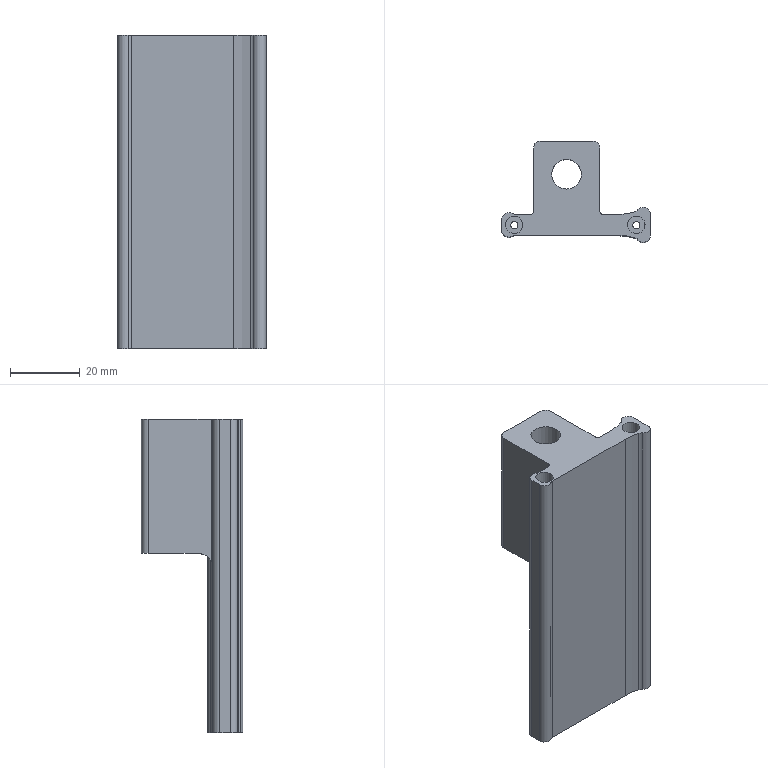Part | NX | features PU-13 2 | 1 solid | 34 faces | box 42.598 x 29.017 x 90 mm | volume 33900 mm3 | cylinder 19 | plane 13 | spline 2 | commonest cylinder face diameters 4 x10 2 x2 2.101 x2 5 x2 8.506 x1 10 x1
STEP:
#1=CARTESIAN_POINT('',(3882.334,-855.122,945.716));
#2=VERTEX_POINT('',#1);
#3=CARTESIAN_POINT('',(3882.334,-855.122,902.217));
#4=VERTEX_POINT('',#3);
#5=CARTESIAN_POINT('',(3882.334,-855.122,935.716));
#6=DIRECTION('',(0.,0.,-1.));
#7=VECTOR('',#6,1000.);
#8=LINE('',#5,#7);
#9=EDGE_CURVE('',#2,#4,#8,.T.);
#10=ORIENTED_EDGE('',*,*,#9,.T.);
#11=CARTESIAN_POINT('',(3903.334,-855.122,902.217));
#12=VERTEX_POINT('',#11);
#13=CARTESIAN_POINT('',(3903.334,-855.122,902.217));
#14=DIRECTION('',(-1.,0.,0.));
#15=VECTOR('',#14,1000.);
#16=LINE('',#13,#15);
#17=EDGE_CURVE('',#4,#12,#16,.F.);
#18=ORIENTED_EDGE('',*,*,#17,.T.);
#19=CARTESIAN_POINT('',(3903.334,-855.122,945.716));
#20=VERTEX_POINT('',#19);
#21=CARTESIAN_POINT('',(3903.334,-855.122,935.716));
#22=DIRECTION('',(0.,0.,-1.));
#23=VECTOR('',#22,1000.);
#24=LINE('',#21,#23);
#25=EDGE_CURVE('',#12,#20,#24,.F.);
#26=ORIENTED_EDGE('',*,*,#25,.T.);
#27=CARTESIAN_POINT('',(3907.495,-855.122,945.716));
#28=VERTEX_POINT('',#27);
#29=CARTESIAN_POINT('',(3897.665,-855.122,945.716));
#30=DIRECTION('',(1.,0.,0.));
#31=VECTOR('',#30,1000.);
#32=LINE('',#29,#31);
#33=EDGE_CURVE('',#20,#28,#32,.T.);
#34=ORIENTED_EDGE('',*,*,#33,.T.);
#35=CARTESIAN_POINT('',(3907.495,-855.122,855.716));
#36=VERTEX_POINT('',#35);
#37=CARTESIAN_POINT('',(3907.495,-855.122,945.716));
#38=CARTESIAN_POINT('',(3907.495,-855.122,915.716));
#39=CARTESIAN_POINT('',(3907.495,-855.122,885.716));
#40=CARTESIAN_POINT('',(3907.495,-855.122,855.716));
#41=B_SPLINE_CURVE_WITH_KNOTS('',3,(#37,#38,#39,#40),.UNSPECIFIED.,.F.,.F.,(4,4),(-0.125,1.),.UNSPECIFIED.);
#42=EDGE_CURVE('',#28,#36,#41,.T.);
#43=ORIENTED_EDGE('',*,*,#42,.T.);
#44=CARTESIAN_POINT('',(3878.173,-855.122,855.716));
#45=VERTEX_POINT('',#44);
#46=CARTESIAN_POINT('',(3897.665,-855.122,855.716));
#47=DIRECTION('',(1.,0.,0.));
#48=VECTOR('',#47,1000.);
#49=LINE('',#46,#48);
#50=EDGE_CURVE('',#36,#45,#49,.F.);
#51=ORIENTED_EDGE('',*,*,#50,.T.);
#52=CARTESIAN_POINT('',(3878.173,-855.122,945.716));
#53=VERTEX_POINT('',#52);
#54=CARTESIAN_POINT('',(3878.173,-855.122,935.716));
#55=DIRECTION('',(0.,0.,-1.));
#56=VECTOR('',#55,1000.);
#57=LINE('',#54,#56);
#58=EDGE_CURVE('',#53,#45,#57,.T.);
#59=ORIENTED_EDGE('',*,*,#58,.F.);
#60=CARTESIAN_POINT('',(3897.665,-855.122,945.716));
#61=DIRECTION('',(1.,0.,0.));
#62=VECTOR('',#61,1000.);
#63=LINE('',#60,#62);
#64=EDGE_CURVE('',#53,#2,#63,.T.);
#65=ORIENTED_EDGE('',*,*,#64,.T.);
#66=EDGE_LOOP('',(#10,#18,#26,#34,#43,#51,#59,#65));
#67=FACE_BOUND('',#66,.T.);
#68=CARTESIAN_POINT('',(3892.84,-855.122,895.716));
#69=DIRECTION('',(0.,1.,0.));
#70=DIRECTION('',(0.,0.,1.));
#71=AXIS2_PLACEMENT_3D('',#68,#69,#70);
#72=PLANE('',#71);
#73=ADVANCED_FACE('',(#67),#72,.T.);
#74=CARTESIAN_POINT('',(3874.236,-856.622,855.716));
#75=VERTEX_POINT('',#74);
#76=CARTESIAN_POINT('',(3874.236,-859.622,855.716));
#77=VERTEX_POINT('',#76);
#78=CARTESIAN_POINT('',(3874.236,-859.622,855.716));
#79=DIRECTION('',(0.,-1.,0.));
#80=VECTOR('',#79,1000.);
#81=LINE('',#78,#80);
#82=EDGE_CURVE('',#75,#77,#81,.T.);
#83=ORIENTED_EDGE('',*,*,#82,.T.);
#84=CARTESIAN_POINT('',(3874.236,-859.622,945.716));
#85=VERTEX_POINT('',#84);
#86=CARTESIAN_POINT('',(3874.236,-859.622,935.716));
#87=DIRECTION('',(0.,0.,-1.));
#88=VECTOR('',#87,1000.);
#89=LINE('',#86,#88);
#90=EDGE_CURVE('',#85,#77,#89,.T.);
#91=ORIENTED_EDGE('',*,*,#90,.F.);
#92=CARTESIAN_POINT('',(3874.236,-856.622,945.716));
#93=VERTEX_POINT('',#92);
#94=CARTESIAN_POINT('',(3874.236,-859.622,945.716));
#95=DIRECTION('',(0.,-1.,0.));
#96=VECTOR('',#95,1000.);
#97=LINE('',#94,#96);
#98=EDGE_CURVE('',#93,#85,#97,.T.);
#99=ORIENTED_EDGE('',*,*,#98,.F.);
#100=CARTESIAN_POINT('',(3874.236,-856.622,945.716));
#101=CARTESIAN_POINT('',(3874.236,-856.622,915.716));
#102=CARTESIAN_POINT('',(3874.236,-856.622,885.716));
#103=CARTESIAN_POINT('',(3874.236,-856.622,855.716));
#104=B_SPLINE_CURVE_WITH_KNOTS('',3,(#100,#101,#102,#103),.UNSPECIFIED.,.F.,.F.,(4,4),(-0.125,1.),.UNSPECIFIED.);
#105=EDGE_CURVE('',#93,#75,#104,.T.);
#106=ORIENTED_EDGE('',*,*,#105,.T.);
#107=EDGE_LOOP('',(#83,#91,#99,#106));
#108=FACE_BOUND('',#107,.T.);
#109=CARTESIAN_POINT('',(3874.236,-859.622,935.716));
#110=DIRECTION('',(1.,0.,0.));
#111=DIRECTION('',(0.,0.,-1.));
#112=AXIS2_PLACEMENT_3D('',#109,#110,#111);
#113=PLANE('',#112);
#114=ADVANCED_FACE('',(#108),#113,.F.);
#115=CARTESIAN_POINT('',(3877.204,-861.372,855.716));
#116=VERTEX_POINT('',#115);
#117=CARTESIAN_POINT('',(3876.236,-859.622,855.716));
#118=DIRECTION('',(0.,0.,1.));
#119=DIRECTION('',(1.,0.,0.));
#120=AXIS2_PLACEMENT_3D('',#117,#118,#119);
#121=CIRCLE('',#120,2.);
#122=EDGE_CURVE('',#116,#77,#121,.F.);
#123=ORIENTED_EDGE('',*,*,#122,.F.);
#124=CARTESIAN_POINT('',(3877.204,-861.372,945.716));
#125=VERTEX_POINT('',#124);
#126=CARTESIAN_POINT('',(3877.204,-861.372,855.716));
#127=CARTESIAN_POINT('',(3877.204,-861.372,885.716));
#128=CARTESIAN_POINT('',(3877.204,-861.372,915.716));
#129=CARTESIAN_POINT('',(3877.204,-861.372,945.716));
#130=B_SPLINE_CURVE_WITH_KNOTS('',3,(#126,#127,#128,#129),.UNSPECIFIED.,.F.,.F.,(4,4),(0.,1.125),.UNSPECIFIED.);
#131=EDGE_CURVE('',#125,#116,#130,.F.);
#132=ORIENTED_EDGE('',*,*,#131,.F.);
#133=CARTESIAN_POINT('',(3876.236,-859.622,945.716));
#134=DIRECTION('',(0.,0.,1.));
#135=DIRECTION('',(1.,0.,0.));
#136=AXIS2_PLACEMENT_3D('',#133,#134,#135);
#137=CIRCLE('',#136,2.);
#138=EDGE_CURVE('',#125,#85,#137,.F.);
#139=ORIENTED_EDGE('',*,*,#138,.T.);
#140=ORIENTED_EDGE('',*,*,#90,.T.);
#141=EDGE_LOOP('',(#123,#132,#139,#140));
#142=FACE_BOUND('',#141,.T.);
#143=CARTESIAN_POINT('',(3876.236,-859.622,935.716));
#144=DIRECTION('',(0.,0.,-1.));
#145=DIRECTION('',(-1.,0.,0.));
#146=AXIS2_PLACEMENT_3D('',#143,#144,#145);
#147=CYLINDRICAL_SURFACE('',#146,2.);
#148=ADVANCED_FACE('',(#142),#147,.T.);
#149=CARTESIAN_POINT('',(3878.173,-861.122,855.716));
#150=VERTEX_POINT('',#149);
#151=CARTESIAN_POINT('',(3878.173,-863.122,855.716));
#152=DIRECTION('',(0.,0.,1.));
#153=DIRECTION('',(1.,0.,0.));
#154=AXIS2_PLACEMENT_3D('',#151,#152,#153);
#155=CIRCLE('',#154,2.);
#156=EDGE_CURVE('',#150,#116,#155,.T.);
#157=ORIENTED_EDGE('',*,*,#156,.F.);
#158=CARTESIAN_POINT('',(3878.173,-861.122,945.716));
#159=VERTEX_POINT('',#158);
#160=CARTESIAN_POINT('',(3878.173,-861.122,935.716));
#161=DIRECTION('',(0.,0.,-1.));
#162=VECTOR('',#161,1000.);
#163=LINE('',#160,#162);
#164=EDGE_CURVE('',#159,#150,#163,.T.);
#165=ORIENTED_EDGE('',*,*,#164,.F.);
#166=CARTESIAN_POINT('',(3878.173,-863.122,945.716));
#167=DIRECTION('',(0.,0.,1.));
#168=DIRECTION('',(1.,0.,0.));
#169=AXIS2_PLACEMENT_3D('',#166,#167,#168);
#170=CIRCLE('',#169,2.);
#171=EDGE_CURVE('',#159,#125,#170,.T.);
#172=ORIENTED_EDGE('',*,*,#171,.T.);
#173=ORIENTED_EDGE('',*,*,#131,.T.);
#174=EDGE_LOOP('',(#157,#165,#172,#173));
#175=FACE_BOUND('',#174,.T.);
#176=CARTESIAN_POINT('',(3878.173,-863.122,935.716));
#177=DIRECTION('',(0.,0.,-1.));
#178=DIRECTION('',(-1.,0.,0.));
#179=AXIS2_PLACEMENT_3D('',#176,#177,#178);
#180=CYLINDRICAL_SURFACE('',#179,2.);
#181=ADVANCED_FACE('',(#175),#180,.F.);
#182=CARTESIAN_POINT('',(3907.495,-861.122,855.716));
#183=VERTEX_POINT('',#182);
#184=CARTESIAN_POINT('',(3897.665,-861.122,855.716));
#185=DIRECTION('',(1.,0.,0.));
#186=VECTOR('',#185,1000.);
#187=LINE('',#184,#186);
#188=EDGE_CURVE('',#150,#183,#187,.T.);
#189=ORIENTED_EDGE('',*,*,#188,.T.);
#190=CARTESIAN_POINT('',(3907.495,-861.122,945.716));
#191=VERTEX_POINT('',#190);
#192=CARTESIAN_POINT('',(3907.495,-861.122,855.716));
#193=CARTESIAN_POINT('',(3907.495,-861.122,885.716));
#194=CARTESIAN_POINT('',(3907.495,-861.122,915.716));
#195=CARTESIAN_POINT('',(3907.495,-861.122,945.716));
#196=B_SPLINE_CURVE_WITH_KNOTS('',3,(#192,#193,#194,#195),.UNSPECIFIED.,.F.,.F.,(4,4),(0.,1.125),.UNSPECIFIED.);
#197=EDGE_CURVE('',#191,#183,#196,.F.);
#198=ORIENTED_EDGE('',*,*,#197,.F.);
#199=CARTESIAN_POINT('',(3897.665,-861.122,945.716));
#200=DIRECTION('',(1.,0.,0.));
#201=VECTOR('',#200,1000.);
#202=LINE('',#199,#201);
#203=EDGE_CURVE('',#159,#191,#202,.T.);
#204=ORIENTED_EDGE('',*,*,#203,.F.);
#205=ORIENTED_EDGE('',*,*,#164,.T.);
#206=EDGE_LOOP('',(#189,#198,#204,#205));
#207=FACE_BOUND('',#206,.T.);
#208=CARTESIAN_POINT('',(3897.665,-861.122,935.716));
#209=DIRECTION('',(0.,1.,0.));
#210=DIRECTION('',(-1.,0.,0.));
#211=AXIS2_PLACEMENT_3D('',#208,#209,#210);
#212=PLANE('',#211);
#213=ADVANCED_FACE('',(#207),#212,.F.);
#214=CARTESIAN_POINT('',(3912.373,-861.817,855.716));
#215=VERTEX_POINT('',#214);
#216=CARTESIAN_POINT('',(3907.495,-861.123,855.716));
#217=CARTESIAN_POINT('',(3909.152,-861.102,855.716));
#218=CARTESIAN_POINT('',(3910.797,-861.337,855.716));
#219=CARTESIAN_POINT('',(3912.373,-861.817,855.716));
#220=B_SPLINE_CURVE_WITH_KNOTS('',3,(#216,#217,#218,#219),.UNSPECIFIED.,.F.,.F.,(4,4),(0.000000834,0.6038),.UNSPECIFIED.);
#221=EDGE_CURVE('',#183,#215,#220,.T.);
#222=ORIENTED_EDGE('',*,*,#221,.T.);
#223=CARTESIAN_POINT('',(3912.373,-861.817,945.716));
#224=VERTEX_POINT('',#223);
#225=CARTESIAN_POINT('',(3912.373,-861.818,945.716));
#226=CARTESIAN_POINT('',(3912.373,-861.818,915.716));
#227=CARTESIAN_POINT('',(3912.373,-861.818,885.716));
#228=CARTESIAN_POINT('',(3912.373,-861.818,855.716));
#229=B_SPLINE_CURVE_WITH_KNOTS('',3,(#225,#226,#227,#228),.UNSPECIFIED.,.F.,.F.,(4,4),(-0.125,1.),.UNSPECIFIED.);
#230=EDGE_CURVE('',#224,#215,#229,.T.);
#231=ORIENTED_EDGE('',*,*,#230,.F.);
#232=CARTESIAN_POINT('',(3912.373,-861.817,945.716));
#233=CARTESIAN_POINT('',(3910.782,-861.333,945.716));
#234=CARTESIAN_POINT('',(3909.156,-861.101,945.716));
#235=CARTESIAN_POINT('',(3907.495,-861.123,945.716));
#236=B_SPLINE_CURVE_WITH_KNOTS('',3,(#232,#233,#234,#235),.UNSPECIFIED.,.F.,.F.,(4,4),(0.,1.),.UNSPECIFIED.);
#237=EDGE_CURVE('',#191,#224,#236,.F.);
#238=ORIENTED_EDGE('',*,*,#237,.F.);
#239=ORIENTED_EDGE('',*,*,#197,.T.);
#240=EDGE_LOOP('',(#222,#231,#238,#239));
#241=FACE_BOUND('',#240,.T.);
#242=CARTESIAN_POINT('',(3907.495,-861.123,945.716));
#243=CARTESIAN_POINT('',(3907.495,-861.123,855.716));
#244=CARTESIAN_POINT('',(3909.152,-861.102,945.716));
#245=CARTESIAN_POINT('',(3909.152,-861.102,855.716));
#246=CARTESIAN_POINT('',(3910.797,-861.337,945.716));
#247=CARTESIAN_POINT('',(3910.797,-861.337,855.716));
#248=CARTESIAN_POINT('',(3912.373,-861.817,945.716));
#249=CARTESIAN_POINT('',(3912.373,-861.817,855.716));
#250=B_SPLINE_SURFACE_WITH_KNOTS('',3,1,((#242,#243),(#244,#245),(#246,#247),(#248,#249)),.SURF_OF_LINEAR_EXTRUSION.,.F.,.F.,.F.,(4,4),(2,2),(0.,0.6038),(0.,1.),.PIECEWISE_BEZIER_KNOTS.);
#251=ADVANCED_FACE('',(#241),#250,.F.);
#252=CARTESIAN_POINT('',(3913.311,-862.434,855.716));
#253=VERTEX_POINT('',#252);
#254=CARTESIAN_POINT('',(3911.787,-863.73,855.716));
#255=DIRECTION('',(0.,0.,1.));
#256=DIRECTION('',(1.,0.,0.));
#257=AXIS2_PLACEMENT_3D('',#254,#255,#256);
#258=CIRCLE('',#257,2.);
#259=EDGE_CURVE('',#215,#253,#258,.F.);
#260=ORIENTED_EDGE('',*,*,#259,.T.);
#261=CARTESIAN_POINT('',(3913.311,-862.434,945.716));
#262=VERTEX_POINT('',#261);
#263=CARTESIAN_POINT('',(3913.311,-862.434,935.716));
#264=DIRECTION('',(0.,0.,-1.));
#265=VECTOR('',#264,1000.);
#266=LINE('',#263,#265);
#267=EDGE_CURVE('',#262,#253,#266,.T.);
#268=ORIENTED_EDGE('',*,*,#267,.F.);
#269=CARTESIAN_POINT('',(3911.787,-863.73,945.716));
#270=DIRECTION('',(0.,0.,1.));
#271=DIRECTION('',(1.,0.,0.));
#272=AXIS2_PLACEMENT_3D('',#269,#270,#271);
#273=CIRCLE('',#272,2.);
#274=EDGE_CURVE('',#224,#262,#273,.F.);
#275=ORIENTED_EDGE('',*,*,#274,.F.);
#276=ORIENTED_EDGE('',*,*,#230,.T.);
#277=EDGE_LOOP('',(#260,#268,#275,#276));
#278=FACE_BOUND('',#277,.T.);
#279=CARTESIAN_POINT('',(3911.787,-863.73,935.716));
#280=DIRECTION('',(0.,0.,-1.));
#281=DIRECTION('',(-1.,0.,0.));
#282=AXIS2_PLACEMENT_3D('',#279,#280,#281);
#283=CYLINDRICAL_SURFACE('',#282,2.);
#284=ADVANCED_FACE('',(#278),#283,.F.);
#285=CARTESIAN_POINT('',(3916.835,-861.139,855.716));
#286=VERTEX_POINT('',#285);
#287=CARTESIAN_POINT('',(3914.835,-861.139,855.716));
#288=DIRECTION('',(0.,0.,1.));
#289=DIRECTION('',(1.,0.,0.));
#290=AXIS2_PLACEMENT_3D('',#287,#288,#289);
#291=CIRCLE('',#290,2.);
#292=EDGE_CURVE('',#286,#253,#291,.F.);
#293=ORIENTED_EDGE('',*,*,#292,.F.);
#294=CARTESIAN_POINT('',(3916.835,-861.139,945.716));
#295=VERTEX_POINT('',#294);
#296=CARTESIAN_POINT('',(3916.835,-861.139,935.716));
#297=DIRECTION('',(0.,0.,-1.));
#298=VECTOR('',#297,1000.);
#299=LINE('',#296,#298);
#300=EDGE_CURVE('',#295,#286,#299,.T.);
#301=ORIENTED_EDGE('',*,*,#300,.F.);
#302=CARTESIAN_POINT('',(3914.835,-861.139,945.716));
#303=DIRECTION('',(0.,0.,1.));
#304=DIRECTION('',(1.,0.,0.));
#305=AXIS2_PLACEMENT_3D('',#302,#303,#304);
#306=CIRCLE('',#305,2.);
#307=EDGE_CURVE('',#295,#262,#306,.F.);
#308=ORIENTED_EDGE('',*,*,#307,.T.);
#309=ORIENTED_EDGE('',*,*,#267,.T.);
#310=EDGE_LOOP('',(#293,#301,#308,#309));
#311=FACE_BOUND('',#310,.T.);
#312=CARTESIAN_POINT('',(3914.835,-861.139,935.716));
#313=DIRECTION('',(0.,0.,-1.));
#314=DIRECTION('',(-1.,0.,0.));
#315=AXIS2_PLACEMENT_3D('',#312,#313,#314);
#316=CYLINDRICAL_SURFACE('',#315,2.);
#317=ADVANCED_FACE('',(#311),#316,.T.);
#318=CARTESIAN_POINT('',(3912.373,-854.427,945.716));
#319=VERTEX_POINT('',#318);
#320=CARTESIAN_POINT('',(3907.495,-855.121,945.716));
#321=CARTESIAN_POINT('',(3909.155,-855.143,945.716));
#322=CARTESIAN_POINT('',(3910.781,-854.911,945.716));
#323=CARTESIAN_POINT('',(3912.373,-854.427,945.716));
#324=B_SPLINE_CURVE_WITH_KNOTS('',3,(#320,#321,#322,#323),.UNSPECIFIED.,.F.,.F.,(4,4),(0.000001378,1.),.UNSPECIFIED.);
#325=EDGE_CURVE('',#28,#319,#324,.T.);
#326=ORIENTED_EDGE('',*,*,#325,.T.);
#327=CARTESIAN_POINT('',(3912.373,-854.427,855.716));
#328=VERTEX_POINT('',#327);
#329=CARTESIAN_POINT('',(3912.373,-854.427,855.716));
#330=CARTESIAN_POINT('',(3912.373,-854.427,885.716));
#331=CARTESIAN_POINT('',(3912.373,-854.427,915.716));
#332=CARTESIAN_POINT('',(3912.373,-854.427,945.716));
#333=B_SPLINE_CURVE_WITH_KNOTS('',3,(#329,#330,#331,#332),.UNSPECIFIED.,.F.,.F.,(4,4),(0.,1.125),.UNSPECIFIED.);
#334=EDGE_CURVE('',#319,#328,#333,.F.);
#335=ORIENTED_EDGE('',*,*,#334,.T.);
#336=CARTESIAN_POINT('',(3912.373,-854.427,855.716));
#337=CARTESIAN_POINT('',(3910.796,-854.907,855.716));
#338=CARTESIAN_POINT('',(3909.152,-855.143,855.716));
#339=CARTESIAN_POINT('',(3907.495,-855.121,855.716));
#340=B_SPLINE_CURVE_WITH_KNOTS('',3,(#336,#337,#338,#339),.UNSPECIFIED.,.F.,.F.,(4,4),(0.3963,1.),.UNSPECIFIED.);
#341=EDGE_CURVE('',#36,#328,#340,.F.);
#342=ORIENTED_EDGE('',*,*,#341,.F.);
#343=ORIENTED_EDGE('',*,*,#42,.F.);
#344=EDGE_LOOP('',(#326,#335,#342,#343));
#345=FACE_BOUND('',#344,.T.);
#346=CARTESIAN_POINT('',(3912.373,-854.427,945.716));
#347=CARTESIAN_POINT('',(3912.373,-854.427,855.716));
#348=CARTESIAN_POINT('',(3910.796,-854.907,945.716));
#349=CARTESIAN_POINT('',(3910.796,-854.907,855.716));
#350=CARTESIAN_POINT('',(3909.152,-855.143,945.716));
#351=CARTESIAN_POINT('',(3909.152,-855.143,855.716));
#352=CARTESIAN_POINT('',(3907.495,-855.121,945.716));
#353=CARTESIAN_POINT('',(3907.495,-855.121,855.716));
#354=B_SPLINE_SURFACE_WITH_KNOTS('',3,1,((#346,#347),(#348,#349),(#350,#351),(#352,#353)),.SURF_OF_LINEAR_EXTRUSION.,.F.,.F.,.F.,(4,4),(2,2),(0.3963,1.),(0.,1.),.PIECEWISE_BEZIER_KNOTS.);
#355=ADVANCED_FACE('',(#345),#354,.F.);
#356=CARTESIAN_POINT('',(3878.885,-858.122,855.716));
#357=VERTEX_POINT('',#356);
#358=CARTESIAN_POINT('',(3877.835,-858.122,855.716));
#359=DIRECTION('',(0.,0.,1.));
#360=DIRECTION('',(1.,0.,0.));
#361=AXIS2_PLACEMENT_3D('',#358,#359,#360);
#362=CIRCLE('',#361,1.05);
#363=EDGE_CURVE('',#357,#357,#362,.T.);
#364=ORIENTED_EDGE('',*,*,#363,.T.);
#365=EDGE_LOOP('',(#364));
#366=FACE_BOUND('',#365,.T.);
#367=CARTESIAN_POINT('',(3913.885,-858.122,855.716));
#368=VERTEX_POINT('',#367);
#369=CARTESIAN_POINT('',(3912.835,-858.122,855.716));
#370=DIRECTION('',(0.,0.,1.));
#371=DIRECTION('',(1.,0.,0.));
#372=AXIS2_PLACEMENT_3D('',#369,#370,#371);
#373=CIRCLE('',#372,1.05);
#374=EDGE_CURVE('',#368,#368,#373,.T.);
#375=ORIENTED_EDGE('',*,*,#374,.T.);
#376=EDGE_LOOP('',(#375));
#377=FACE_BOUND('',#376,.T.);
#378=ORIENTED_EDGE('',*,*,#341,.T.);
#379=CARTESIAN_POINT('',(3913.311,-853.81,855.716));
#380=VERTEX_POINT('',#379);
#381=CARTESIAN_POINT('',(3911.787,-852.514,855.716));
#382=DIRECTION('',(0.,0.,1.));
#383=DIRECTION('',(1.,0.,0.));
#384=AXIS2_PLACEMENT_3D('',#381,#382,#383);
#385=CIRCLE('',#384,2.);
#386=EDGE_CURVE('',#380,#328,#385,.F.);
#387=ORIENTED_EDGE('',*,*,#386,.F.);
#388=CARTESIAN_POINT('',(3916.835,-855.105,855.716));
#389=VERTEX_POINT('',#388);
#390=CARTESIAN_POINT('',(3914.835,-855.105,855.716));
#391=DIRECTION('',(0.,0.,1.));
#392=DIRECTION('',(1.,0.,0.));
#393=AXIS2_PLACEMENT_3D('',#390,#391,#392);
#394=CIRCLE('',#393,2.);
#395=EDGE_CURVE('',#389,#380,#394,.T.);
#396=ORIENTED_EDGE('',*,*,#395,.F.);
#397=CARTESIAN_POINT('',(3916.835,-859.622,855.716));
#398=DIRECTION('',(0.,-1.,0.));
#399=VECTOR('',#398,1000.);
#400=LINE('',#397,#399);
#401=EDGE_CURVE('',#286,#389,#400,.F.);
#402=ORIENTED_EDGE('',*,*,#401,.F.);
#403=ORIENTED_EDGE('',*,*,#292,.T.);
#404=ORIENTED_EDGE('',*,*,#259,.F.);
#405=ORIENTED_EDGE('',*,*,#221,.F.);
#406=ORIENTED_EDGE('',*,*,#188,.F.);
#407=ORIENTED_EDGE('',*,*,#156,.T.);
#408=ORIENTED_EDGE('',*,*,#122,.T.);
#409=ORIENTED_EDGE('',*,*,#82,.F.);
#410=CARTESIAN_POINT('',(3877.204,-854.872,855.716));
#411=VERTEX_POINT('',#410);
#412=CARTESIAN_POINT('',(3876.236,-856.622,855.716));
#413=DIRECTION('',(0.,0.,1.));
#414=DIRECTION('',(1.,0.,0.));
#415=AXIS2_PLACEMENT_3D('',#412,#413,#414);
#416=CIRCLE('',#415,2.);
#417=EDGE_CURVE('',#75,#411,#416,.F.);
#418=ORIENTED_EDGE('',*,*,#417,.T.);
#419=CARTESIAN_POINT('',(3878.173,-853.122,855.716));
#420=DIRECTION('',(0.,0.,1.));
#421=DIRECTION('',(1.,0.,0.));
#422=AXIS2_PLACEMENT_3D('',#419,#420,#421);
#423=CIRCLE('',#422,2.);
#424=EDGE_CURVE('',#411,#45,#423,.T.);
#425=ORIENTED_EDGE('',*,*,#424,.T.);
#426=ORIENTED_EDGE('',*,*,#50,.F.);
#427=EDGE_LOOP('',(#378,#387,#396,#402,#403,#404,#405,#406,#407,#408,#409,#418,#425,#426));
#428=FACE_BOUND('',#427,.T.);
#429=CARTESIAN_POINT('',(3897.665,-859.622,855.716));
#430=DIRECTION('',(0.,0.,1.));
#431=DIRECTION('',(1.,0.,0.));
#432=AXIS2_PLACEMENT_3D('',#429,#430,#431);
#433=PLANE('',#432);
#434=ADVANCED_FACE('',(#366,#377,#428),#433,.F.);
#435=CARTESIAN_POINT('',(3880.335,-858.122,945.716));
#436=VERTEX_POINT('',#435);
#437=CARTESIAN_POINT('',(3877.835,-858.122,945.716));
#438=DIRECTION('',(0.,0.,1.));
#439=DIRECTION('',(1.,0.,0.));
#440=AXIS2_PLACEMENT_3D('',#437,#438,#439);
#441=CIRCLE('',#440,2.5);
#442=EDGE_CURVE('',#436,#436,#441,.F.);
#443=ORIENTED_EDGE('',*,*,#442,.T.);
#444=EDGE_LOOP('',(#443));
#445=FACE_BOUND('',#444,.T.);
#446=CARTESIAN_POINT('',(3915.335,-858.122,945.716));
#447=VERTEX_POINT('',#446);
#448=CARTESIAN_POINT('',(3912.835,-858.122,945.716));
#449=DIRECTION('',(0.,0.,1.));
#450=DIRECTION('',(1.,0.,0.));
#451=AXIS2_PLACEMENT_3D('',#448,#449,#450);
#452=CIRCLE('',#451,2.5);
#453=EDGE_CURVE('',#447,#447,#452,.F.);
#454=ORIENTED_EDGE('',*,*,#453,.T.);
#455=EDGE_LOOP('',(#454));
#456=FACE_BOUND('',#455,.T.);
#457=CARTESIAN_POINT('',(3916.835,-855.105,945.716));
#458=VERTEX_POINT('',#457);
#459=CARTESIAN_POINT('',(3916.835,-859.622,945.716));
#460=DIRECTION('',(0.,-1.,0.));
#461=VECTOR('',#460,1000.);
#462=LINE('',#459,#461);
#463=EDGE_CURVE('',#295,#458,#462,.F.);
#464=ORIENTED_EDGE('',*,*,#463,.T.);
#465=CARTESIAN_POINT('',(3913.311,-853.81,945.716));
#466=VERTEX_POINT('',#465);
#467=CARTESIAN_POINT('',(3914.835,-855.105,945.716));
#468=DIRECTION('',(0.,0.,1.));
#469=DIRECTION('',(1.,0.,0.));
#470=AXIS2_PLACEMENT_3D('',#467,#468,#469);
#471=CIRCLE('',#470,2.);
#472=EDGE_CURVE('',#458,#466,#471,.T.);
#473=ORIENTED_EDGE('',*,*,#472,.T.);
#474=CARTESIAN_POINT('',(3911.787,-852.514,945.716));
#475=DIRECTION('',(0.,0.,1.));
#476=DIRECTION('',(1.,0.,0.));
#477=AXIS2_PLACEMENT_3D('',#474,#475,#476);
#478=CIRCLE('',#477,2.);
#479=EDGE_CURVE('',#466,#319,#478,.F.);
#480=ORIENTED_EDGE('',*,*,#479,.T.);
#481=ORIENTED_EDGE('',*,*,#325,.F.);
#482=ORIENTED_EDGE('',*,*,#33,.F.);
#483=CARTESIAN_POINT('',(3902.334,-854.122,945.716));
#484=VERTEX_POINT('',#483);
#485=CARTESIAN_POINT('',(3903.334,-854.122,945.716));
#486=DIRECTION('',(0.,0.,1.));
#487=DIRECTION('',(1.,0.,0.));
#488=AXIS2_PLACEMENT_3D('',#485,#486,#487);
#489=CIRCLE('',#488,1.);
#490=EDGE_CURVE('',#20,#484,#489,.F.);
#491=ORIENTED_EDGE('',*,*,#490,.T.);
#492=CARTESIAN_POINT('',(3902.334,-836.122,945.716));
#493=VERTEX_POINT('',#492);
#494=CARTESIAN_POINT('',(3902.334,-855.122,945.716));
#495=DIRECTION('',(0.,-1.,0.));
#496=VECTOR('',#495,1000.);
#497=LINE('',#494,#496);
#498=EDGE_CURVE('',#493,#484,#497,.T.);
#499=ORIENTED_EDGE('',*,*,#498,.F.);
#500=CARTESIAN_POINT('',(3900.334,-834.122,945.716));
#501=VERTEX_POINT('',#500);
#502=CARTESIAN_POINT('',(3900.334,-836.122,945.716));
#503=DIRECTION('',(0.,0.,-1.));
#504=DIRECTION('',(0.,-1.,0.));
#505=AXIS2_PLACEMENT_3D('',#502,#503,#504);
#506=CIRCLE('',#505,2.);
#507=EDGE_CURVE('',#493,#501,#506,.F.);
#508=ORIENTED_EDGE('',*,*,#507,.T.);
#509=CARTESIAN_POINT('',(3885.334,-834.122,945.716));
#510=VERTEX_POINT('',#509);
#511=CARTESIAN_POINT('',(3882.759,-834.122,945.716));
#512=DIRECTION('',(1.,0.,0.));
#513=VECTOR('',#512,1000.);
#514=LINE('',#511,#513);
#515=EDGE_CURVE('',#510,#501,#514,.T.);
#516=ORIENTED_EDGE('',*,*,#515,.F.);
#517=CARTESIAN_POINT('',(3883.334,-836.122,945.716));
#518=VERTEX_POINT('',#517);
#519=CARTESIAN_POINT('',(3885.334,-836.122,945.716));
#520=DIRECTION('',(0.,0.,-1.));
#521=DIRECTION('',(0.,-1.,0.));
#522=AXIS2_PLACEMENT_3D('',#519,#520,#521);
#523=CIRCLE('',#522,2.);
#524=EDGE_CURVE('',#510,#518,#523,.F.);
#525=ORIENTED_EDGE('',*,*,#524,.T.);
#526=CARTESIAN_POINT('',(3883.334,-854.122,945.716));
#527=VERTEX_POINT('',#526);
#528=CARTESIAN_POINT('',(3883.334,-855.172,945.716));
#529=DIRECTION('',(0.,1.,0.));
#530=VECTOR('',#529,1000.);
#531=LINE('',#528,#530);
#532=EDGE_CURVE('',#527,#518,#531,.T.);
#533=ORIENTED_EDGE('',*,*,#532,.F.);
#534=CARTESIAN_POINT('',(3882.334,-854.122,945.716));
#535=DIRECTION('',(0.,0.,1.));
#536=DIRECTION('',(1.,0.,0.));
#537=AXIS2_PLACEMENT_3D('',#534,#535,#536);
#538=CIRCLE('',#537,1.);
#539=EDGE_CURVE('',#527,#2,#538,.F.);
#540=ORIENTED_EDGE('',*,*,#539,.T.);
#541=ORIENTED_EDGE('',*,*,#64,.F.);
#542=CARTESIAN_POINT('',(3877.204,-854.872,945.716));
#543=VERTEX_POINT('',#542);
#544=CARTESIAN_POINT('',(3878.173,-853.122,945.716));
#545=DIRECTION('',(0.,0.,1.));
#546=DIRECTION('',(1.,0.,0.));
#547=AXIS2_PLACEMENT_3D('',#544,#545,#546);
#548=CIRCLE('',#547,2.);
#549=EDGE_CURVE('',#543,#53,#548,.T.);
#550=ORIENTED_EDGE('',*,*,#549,.F.);
#551=CARTESIAN_POINT('',(3876.236,-856.622,945.716));
#552=DIRECTION('',(0.,0.,1.));
#553=DIRECTION('',(1.,0.,0.));
#554=AXIS2_PLACEMENT_3D('',#551,#552,#553);
#555=CIRCLE('',#554,2.);
#556=EDGE_CURVE('',#93,#543,#555,.F.);
#557=ORIENTED_EDGE('',*,*,#556,.F.);
#558=ORIENTED_EDGE('',*,*,#98,.T.);
#559=ORIENTED_EDGE('',*,*,#138,.F.);
#560=ORIENTED_EDGE('',*,*,#171,.F.);
#561=ORIENTED_EDGE('',*,*,#203,.T.);
#562=ORIENTED_EDGE('',*,*,#237,.T.);
#563=ORIENTED_EDGE('',*,*,#274,.T.);
#564=ORIENTED_EDGE('',*,*,#307,.F.);
#565=EDGE_LOOP('',(#464,#473,#480,#481,#482,#491,#499,#508,#516,#525,#533,#540,#541,#550,#557,#558,#559,#560,#561,#562,#563,#564));
#566=FACE_BOUND('',#565,.T.);
#567=CARTESIAN_POINT('',(3892.834,-847.875,945.716));
#568=VERTEX_POINT('',#567);
#569=CARTESIAN_POINT('',(3892.834,-843.622,945.716));
#570=DIRECTION('',(0.,0.,-1.));
#571=DIRECTION('',(0.,-1.,0.));
#572=AXIS2_PLACEMENT_3D('',#569,#570,#571);
#573=CIRCLE('',#572,4.253);
#574=EDGE_CURVE('',#568,#568,#573,.F.);
#575=ORIENTED_EDGE('',*,*,#574,.F.);
#576=EDGE_LOOP('',(#575));
#577=FACE_BOUND('',#576,.T.);
#578=CARTESIAN_POINT('',(3897.665,-859.622,945.716));
#579=DIRECTION('',(0.,0.,1.));
#580=DIRECTION('',(1.,0.,0.));
#581=AXIS2_PLACEMENT_3D('',#578,#579,#580);
#582=PLANE('',#581);
#583=ADVANCED_FACE('',(#445,#456,#566,#577),#582,.T.);
#584=ORIENTED_EDGE('',*,*,#401,.T.);
#585=CARTESIAN_POINT('',(3916.835,-855.105,935.716));
#586=DIRECTION('',(0.,0.,-1.));
#587=VECTOR('',#586,1000.);
#588=LINE('',#585,#587);
#589=EDGE_CURVE('',#458,#389,#588,.T.);
#590=ORIENTED_EDGE('',*,*,#589,.F.);
#591=ORIENTED_EDGE('',*,*,#463,.F.);
#592=ORIENTED_EDGE('',*,*,#300,.T.);
#593=EDGE_LOOP('',(#584,#590,#591,#592));
#594=FACE_BOUND('',#593,.T.);
#595=CARTESIAN_POINT('',(3916.835,-859.622,935.716));
#596=DIRECTION('',(-1.,0.,0.));
#597=DIRECTION('',(0.,0.,1.));
#598=AXIS2_PLACEMENT_3D('',#595,#596,#597);
#599=PLANE('',#598);
#600=ADVANCED_FACE('',(#594),#599,.F.);
#601=ORIENTED_EDGE('',*,*,#556,.T.);
#602=CARTESIAN_POINT('',(3877.204,-854.872,935.716));
#603=DIRECTION('',(0.,0.,-1.));
#604=VECTOR('',#603,1000.);
#605=LINE('',#602,#604);
#606=EDGE_CURVE('',#543,#411,#605,.T.);
#607=ORIENTED_EDGE('',*,*,#606,.T.);
#608=ORIENTED_EDGE('',*,*,#417,.F.);
#609=ORIENTED_EDGE('',*,*,#105,.F.);
#610=EDGE_LOOP('',(#601,#607,#608,#609));
#611=FACE_BOUND('',#610,.T.);
#612=CARTESIAN_POINT('',(3876.236,-856.622,935.716));
#613=DIRECTION('',(0.,0.,-1.));
#614=DIRECTION('',(-1.,0.,0.));
#615=AXIS2_PLACEMENT_3D('',#612,#613,#614);
#616=CYLINDRICAL_SURFACE('',#615,2.);
#617=ADVANCED_FACE('',(#611),#616,.T.);
#618=ORIENTED_EDGE('',*,*,#424,.F.);
#619=ORIENTED_EDGE('',*,*,#606,.F.);
#620=ORIENTED_EDGE('',*,*,#549,.T.);
#621=ORIENTED_EDGE('',*,*,#58,.T.);
#622=EDGE_LOOP('',(#618,#619,#620,#621));
#623=FACE_BOUND('',#622,.T.);
#624=CARTESIAN_POINT('',(3878.173,-853.122,935.716));
#625=DIRECTION('',(0.,0.,-1.));
#626=DIRECTION('',(-1.,0.,0.));
#627=AXIS2_PLACEMENT_3D('',#624,#625,#626);
#628=CYLINDRICAL_SURFACE('',#627,2.);
#629=ADVANCED_FACE('',(#623),#628,.F.);
#630=CARTESIAN_POINT('',(3902.334,-836.122,907.217));
#631=VERTEX_POINT('',#630);
#632=CARTESIAN_POINT('',(3902.334,-850.122,907.217));
#633=VERTEX_POINT('',#632);
#634=CARTESIAN_POINT('',(3902.334,-720.473,907.217));
#635=DIRECTION('',(0.,-1.,0.));
#636=VECTOR('',#635,1000.);
#637=LINE('',#634,#636);
#638=EDGE_CURVE('',#631,#633,#637,.T.);
#639=ORIENTED_EDGE('',*,*,#638,.T.);
#640=CARTESIAN_POINT('',(3896.045,-850.122,907.217));
#641=VERTEX_POINT('',#640);
#642=CARTESIAN_POINT('',(3882.334,-850.122,907.217));
#643=DIRECTION('',(-1.,0.,0.));
#644=VECTOR('',#643,1000.);
#645=LINE('',#642,#644);
#646=EDGE_CURVE('',#633,#641,#645,.T.);
#647=ORIENTED_EDGE('',*,*,#646,.T.);
#648=CARTESIAN_POINT('',(3889.623,-850.122,907.217));
#649=VERTEX_POINT('',#648);
#650=CARTESIAN_POINT('',(3892.834,-843.622,907.217));
#651=DIRECTION('',(0.,0.,1.));
#652=DIRECTION('',(0.,-1.,0.));
#653=AXIS2_PLACEMENT_3D('',#650,#651,#652);
#654=CIRCLE('',#653,7.25);
#655=EDGE_CURVE('',#641,#649,#654,.T.);
#656=ORIENTED_EDGE('',*,*,#655,.T.);
#657=CARTESIAN_POINT('',(3883.334,-850.122,907.217));
#658=VERTEX_POINT('',#657);
#659=CARTESIAN_POINT('',(3882.334,-850.122,907.217));
#660=DIRECTION('',(-1.,0.,0.));
#661=VECTOR('',#660,1000.);
#662=LINE('',#659,#661);
#663=EDGE_CURVE('',#649,#658,#662,.T.);
#664=ORIENTED_EDGE('',*,*,#663,.T.);
#665=CARTESIAN_POINT('',(3883.334,-836.122,907.217));
#666=VERTEX_POINT('',#665);
#667=CARTESIAN_POINT('',(3883.334,-720.473,907.217));
#668=DIRECTION('',(0.,1.,0.));
#669=VECTOR('',#668,1000.);
#670=LINE('',#667,#669);
#671=EDGE_CURVE('',#658,#666,#670,.T.);
#672=ORIENTED_EDGE('',*,*,#671,.T.);
#673=CARTESIAN_POINT('',(3885.334,-834.122,907.217));
#674=VERTEX_POINT('',#673);
#675=CARTESIAN_POINT('',(3885.334,-836.122,907.217));
#676=DIRECTION('',(0.,0.,-1.));
#677=DIRECTION('',(0.,-1.,0.));
#678=AXIS2_PLACEMENT_3D('',#675,#676,#677);
#679=CIRCLE('',#678,2.);
#680=EDGE_CURVE('',#666,#674,#679,.T.);
#681=ORIENTED_EDGE('',*,*,#680,.T.);
#682=CARTESIAN_POINT('',(3900.334,-834.122,907.217));
#683=VERTEX_POINT('',#682);
#684=CARTESIAN_POINT('',(3146.836,-834.122,907.217));
#685=DIRECTION('',(1.,0.,0.));
#686=VECTOR('',#685,1000.);
#687=LINE('',#684,#686);
#688=EDGE_CURVE('',#674,#683,#687,.T.);
#689=ORIENTED_EDGE('',*,*,#688,.T.);
#690=CARTESIAN_POINT('',(3900.334,-836.122,907.217));
#691=DIRECTION('',(0.,0.,-1.));
#692=DIRECTION('',(0.,-1.,0.));
#693=AXIS2_PLACEMENT_3D('',#690,#691,#692);
#694=CIRCLE('',#693,2.);
#695=EDGE_CURVE('',#683,#631,#694,.T.);
#696=ORIENTED_EDGE('',*,*,#695,.T.);
#697=EDGE_LOOP('',(#639,#647,#656,#664,#672,#681,#689,#696));
#698=FACE_BOUND('',#697,.T.);
#699=CARTESIAN_POINT('',(3146.836,-720.473,907.217));
#700=DIRECTION('',(0.,0.,-1.));
#701=DIRECTION('',(-1.,0.,0.));
#702=AXIS2_PLACEMENT_3D('',#699,#700,#701);
#703=PLANE('',#702);
#704=ADVANCED_FACE('',(#698),#703,.T.);
#705=ORIENTED_EDGE('',*,*,#498,.T.);
#706=CARTESIAN_POINT('',(3902.334,-854.122,905.217));
#707=VERTEX_POINT('',#706);
#708=CARTESIAN_POINT('',(3902.334,-854.122,929.216));
#709=DIRECTION('',(0.,0.,-1.));
#710=VECTOR('',#709,1000.);
#711=LINE('',#708,#710);
#712=EDGE_CURVE('',#484,#707,#711,.T.);
#713=ORIENTED_EDGE('',*,*,#712,.T.);
#714=CARTESIAN_POINT('',(3902.334,-850.122,902.217));
#715=DIRECTION('',(-1.,0.,0.));
#716=DIRECTION('',(0.,-1.,0.));
#717=AXIS2_PLACEMENT_3D('',#714,#715,#716);
#718=CIRCLE('',#717,5.);
#719=EDGE_CURVE('',#707,#633,#718,.T.);
#720=ORIENTED_EDGE('',*,*,#719,.T.);
#721=ORIENTED_EDGE('',*,*,#638,.F.);
#722=CARTESIAN_POINT('',(3902.334,-836.122,929.216));
#723=DIRECTION('',(0.,0.,1.));
#724=VECTOR('',#723,1000.);
#725=LINE('',#722,#724);
#726=EDGE_CURVE('',#631,#493,#725,.T.);
#727=ORIENTED_EDGE('',*,*,#726,.T.);
#728=EDGE_LOOP('',(#705,#713,#720,#721,#727));
#729=FACE_BOUND('',#728,.T.);
#730=CARTESIAN_POINT('',(3902.334,-855.122,929.216));
#731=DIRECTION('',(-1.,0.,0.));
#732=DIRECTION('',(0.,0.,1.));
#733=AXIS2_PLACEMENT_3D('',#730,#731,#732);
#734=PLANE('',#733);
#735=ADVANCED_FACE('',(#729),#734,.F.);
#736=ORIENTED_EDGE('',*,*,#671,.F.);
#737=CARTESIAN_POINT('',(3883.334,-854.122,905.217));
#738=VERTEX_POINT('',#737);
#739=CARTESIAN_POINT('',(3883.334,-850.122,902.217));
#740=DIRECTION('',(1.,0.,0.));
#741=DIRECTION('',(0.,1.,0.));
#742=AXIS2_PLACEMENT_3D('',#739,#740,#741);
#743=CIRCLE('',#742,5.);
#744=EDGE_CURVE('',#658,#738,#743,.T.);
#745=ORIENTED_EDGE('',*,*,#744,.T.);
#746=CARTESIAN_POINT('',(3883.334,-854.122,929.216));
#747=DIRECTION('',(0.,0.,-1.));
#748=VECTOR('',#747,1000.);
#749=LINE('',#746,#748);
#750=EDGE_CURVE('',#738,#527,#749,.F.);
#751=ORIENTED_EDGE('',*,*,#750,.T.);
#752=ORIENTED_EDGE('',*,*,#532,.T.);
#753=CARTESIAN_POINT('',(3883.334,-836.122,929.216));
#754=DIRECTION('',(0.,0.,-1.));
#755=VECTOR('',#754,1000.);
#756=LINE('',#753,#755);
#757=EDGE_CURVE('',#518,#666,#756,.T.);
#758=ORIENTED_EDGE('',*,*,#757,.T.);
#759=EDGE_LOOP('',(#736,#745,#751,#752,#758));
#760=FACE_BOUND('',#759,.T.);
#761=CARTESIAN_POINT('',(3883.334,-855.172,929.216));
#762=DIRECTION('',(1.,0.,0.));
#763=DIRECTION('',(0.,0.,-1.));
#764=AXIS2_PLACEMENT_3D('',#761,#762,#763);
#765=PLANE('',#764);
#766=ADVANCED_FACE('',(#760),#765,.F.);
#767=CARTESIAN_POINT('',(3889.623,-850.122,907.217));
#768=CARTESIAN_POINT('',(3890.626,-850.618,907.217));
#769=CARTESIAN_POINT('',(3892.827,-851.126,907.103));
#770=CARTESIAN_POINT('',(3895.042,-850.618,907.217));
#771=CARTESIAN_POINT('',(3896.045,-850.122,907.217));
#772=B_SPLINE_CURVE_WITH_KNOTS('',3,(#767,#768,#769,#770,#771),.UNSPECIFIED.,.F.,.F.,(4,1,4),(0.,0.003304,0.006609),.UNSPECIFIED.);
#773=EDGE_CURVE('',#649,#641,#772,.T.);
#774=ORIENTED_EDGE('',*,*,#773,.F.);
#775=ORIENTED_EDGE('',*,*,#655,.F.);
#776=EDGE_LOOP('',(#774,#775));
#777=FACE_BOUND('',#776,.T.);
#778=CARTESIAN_POINT('',(3892.834,-836.372,922.216));
#779=VERTEX_POINT('',#778);
#780=CARTESIAN_POINT('',(3892.834,-843.622,922.216));
#781=DIRECTION('',(0.,0.,1.));
#782=DIRECTION('',(1.,0.,0.));
#783=AXIS2_PLACEMENT_3D('',#780,#781,#782);
#784=CIRCLE('',#783,7.25);
#785=EDGE_CURVE('',#779,#779,#784,.F.);
#786=ORIENTED_EDGE('',*,*,#785,.F.);
#787=EDGE_LOOP('',(#786));
#788=FACE_BOUND('',#787,.T.);
#789=CARTESIAN_POINT('',(3892.834,-843.622,912.216));
#790=DIRECTION('',(0.,0.,-1.));
#791=DIRECTION('',(0.,1.,0.));
#792=AXIS2_PLACEMENT_3D('',#789,#790,#791);
#793=CYLINDRICAL_SURFACE('',#792,7.25);
#794=ADVANCED_FACE('',(#777,#788),#793,.F.);
#795=CARTESIAN_POINT('',(3892.834,-839.369,922.216));
#796=VERTEX_POINT('',#795);
#797=CARTESIAN_POINT('',(3892.834,-843.622,922.216));
#798=DIRECTION('',(0.,0.,1.));
#799=DIRECTION('',(1.,0.,0.));
#800=AXIS2_PLACEMENT_3D('',#797,#798,#799);
#801=CIRCLE('',#800,4.253);
#802=EDGE_CURVE('',#796,#796,#801,.T.);
#803=ORIENTED_EDGE('',*,*,#802,.T.);
#804=EDGE_LOOP('',(#803));
#805=FACE_BOUND('',#804,.T.);
#806=ORIENTED_EDGE('',*,*,#785,.T.);
#807=EDGE_LOOP('',(#806));
#808=FACE_BOUND('',#807,.T.);
#809=CARTESIAN_POINT('',(3834.912,-370.591,922.216));
#810=DIRECTION('',(0.,0.,1.));
#811=DIRECTION('',(0.,-1.,0.));
#812=AXIS2_PLACEMENT_3D('',#809,#810,#811);
#813=PLANE('',#812);
#814=ADVANCED_FACE('',(#805,#808),#813,.F.);
#815=ORIENTED_EDGE('',*,*,#574,.T.);
#816=EDGE_LOOP('',(#815));
#817=FACE_BOUND('',#816,.T.);
#818=ORIENTED_EDGE('',*,*,#802,.F.);
#819=EDGE_LOOP('',(#818));
#820=FACE_BOUND('',#819,.T.);
#821=CARTESIAN_POINT('',(3892.834,-843.622,947.216));
#822=DIRECTION('',(0.,0.,-1.));
#823=DIRECTION('',(0.,1.,0.));
#824=AXIS2_PLACEMENT_3D('',#821,#822,#823);
#825=CYLINDRICAL_SURFACE('',#824,4.253);
#826=ADVANCED_FACE('',(#817,#820),#825,.F.);
#827=ORIENTED_EDGE('',*,*,#695,.F.);
#828=CARTESIAN_POINT('',(3900.334,-834.122,929.216));
#829=DIRECTION('',(0.,0.,-1.));
#830=VECTOR('',#829,1000.);
#831=LINE('',#828,#830);
#832=EDGE_CURVE('',#501,#683,#831,.T.);
#833=ORIENTED_EDGE('',*,*,#832,.F.);
#834=ORIENTED_EDGE('',*,*,#507,.F.);
#835=ORIENTED_EDGE('',*,*,#726,.F.);
#836=EDGE_LOOP('',(#827,#833,#834,#835));
#837=FACE_BOUND('',#836,.T.);
#838=CARTESIAN_POINT('',(3900.334,-836.122,929.216));
#839=DIRECTION('',(0.,0.,1.));
#840=DIRECTION('',(0.,-1.,0.));
#841=AXIS2_PLACEMENT_3D('',#838,#839,#840);
#842=CYLINDRICAL_SURFACE('',#841,2.);
#843=ADVANCED_FACE('',(#837),#842,.T.);
#844=ORIENTED_EDGE('',*,*,#515,.T.);
#845=ORIENTED_EDGE('',*,*,#832,.T.);
#846=ORIENTED_EDGE('',*,*,#688,.F.);
#847=CARTESIAN_POINT('',(3885.334,-834.122,929.216));
#848=DIRECTION('',(0.,0.,1.));
#849=VECTOR('',#848,1000.);
#850=LINE('',#847,#849);
#851=EDGE_CURVE('',#674,#510,#850,.T.);
#852=ORIENTED_EDGE('',*,*,#851,.T.);
#853=EDGE_LOOP('',(#844,#845,#846,#852));
#854=FACE_BOUND('',#853,.T.);
#855=CARTESIAN_POINT('',(3882.759,-834.122,929.216));
#856=DIRECTION('',(0.,-1.,0.));
#857=DIRECTION('',(0.,0.,1.));
#858=AXIS2_PLACEMENT_3D('',#855,#856,#857);
#859=PLANE('',#858);
#860=ADVANCED_FACE('',(#854),#859,.F.);
#861=ORIENTED_EDGE('',*,*,#680,.F.);
#862=ORIENTED_EDGE('',*,*,#757,.F.);
#863=ORIENTED_EDGE('',*,*,#524,.F.);
#864=ORIENTED_EDGE('',*,*,#851,.F.);
#865=EDGE_LOOP('',(#861,#862,#863,#864));
#866=FACE_BOUND('',#865,.T.);
#867=CARTESIAN_POINT('',(3885.334,-836.122,929.216));
#868=DIRECTION('',(0.,0.,-1.));
#869=DIRECTION('',(0.,1.,0.));
#870=AXIS2_PLACEMENT_3D('',#867,#868,#869);
#871=CYLINDRICAL_SURFACE('',#870,2.);
#872=ADVANCED_FACE('',(#866),#871,.T.);
#873=ORIENTED_EDGE('',*,*,#539,.F.);
#874=ORIENTED_EDGE('',*,*,#750,.F.);
#875=CARTESIAN_POINT('',(3883.334,-854.122,905.217));
#876=CARTESIAN_POINT('',(3883.334,-854.808,904.301));
#877=CARTESIAN_POINT('',(3882.795,-855.122,903.247));
#878=CARTESIAN_POINT('',(3882.334,-855.122,902.217));
#879=B_SPLINE_CURVE_WITH_KNOTS('',3,(#875,#876,#877,#878),.UNSPECIFIED.,.F.,.F.,(4,4),(0.,0.003386),.UNSPECIFIED.);
#880=EDGE_CURVE('',#738,#4,#879,.T.);
#881=ORIENTED_EDGE('',*,*,#880,.T.);
#882=ORIENTED_EDGE('',*,*,#9,.F.);
#883=EDGE_LOOP('',(#873,#874,#881,#882));
#884=FACE_BOUND('',#883,.T.);
#885=CARTESIAN_POINT('',(3882.334,-854.122,935.716));
#886=DIRECTION('',(0.,0.,-1.));
#887=DIRECTION('',(-1.,0.,0.));
#888=AXIS2_PLACEMENT_3D('',#885,#886,#887);
#889=CYLINDRICAL_SURFACE('',#888,1.);
#890=ADVANCED_FACE('',(#884),#889,.F.);
#891=ORIENTED_EDGE('',*,*,#490,.F.);
#892=ORIENTED_EDGE('',*,*,#25,.F.);
#893=CARTESIAN_POINT('',(3902.334,-854.122,905.217));
#894=CARTESIAN_POINT('',(3902.334,-854.808,904.301));
#895=CARTESIAN_POINT('',(3902.873,-855.122,903.247));
#896=CARTESIAN_POINT('',(3903.334,-855.122,902.217));
#897=B_SPLINE_CURVE_WITH_KNOTS('',3,(#893,#894,#895,#896),.UNSPECIFIED.,.F.,.F.,(4,4),(0.,0.003386),.UNSPECIFIED.);
#898=EDGE_CURVE('',#12,#707,#897,.F.);
#899=ORIENTED_EDGE('',*,*,#898,.T.);
#900=ORIENTED_EDGE('',*,*,#712,.F.);
#901=EDGE_LOOP('',(#891,#892,#899,#900));
#902=FACE_BOUND('',#901,.T.);
#903=CARTESIAN_POINT('',(3903.334,-854.122,929.216));
#904=DIRECTION('',(0.,0.,-1.));
#905=DIRECTION('',(-1.,0.,0.));
#906=AXIS2_PLACEMENT_3D('',#903,#904,#905);
#907=CYLINDRICAL_SURFACE('',#906,1.);
#908=ADVANCED_FACE('',(#902),#907,.F.);
#909=ORIENTED_EDGE('',*,*,#395,.T.);
#910=CARTESIAN_POINT('',(3913.311,-853.81,935.716));
#911=DIRECTION('',(0.,0.,-1.));
#912=VECTOR('',#911,1000.);
#913=LINE('',#910,#912);
#914=EDGE_CURVE('',#466,#380,#913,.T.);
#915=ORIENTED_EDGE('',*,*,#914,.F.);
#916=ORIENTED_EDGE('',*,*,#472,.F.);
#917=ORIENTED_EDGE('',*,*,#589,.T.);
#918=EDGE_LOOP('',(#909,#915,#916,#917));
#919=FACE_BOUND('',#918,.T.);
#920=CARTESIAN_POINT('',(3914.835,-855.105,935.716));
#921=DIRECTION('',(0.,0.,-1.));
#922=DIRECTION('',(-1.,0.,0.));
#923=AXIS2_PLACEMENT_3D('',#920,#921,#922);
#924=CYLINDRICAL_SURFACE('',#923,2.);
#925=ADVANCED_FACE('',(#919),#924,.T.);
#926=ORIENTED_EDGE('',*,*,#386,.T.);
#927=ORIENTED_EDGE('',*,*,#334,.F.);
#928=ORIENTED_EDGE('',*,*,#479,.F.);
#929=ORIENTED_EDGE('',*,*,#914,.T.);
#930=EDGE_LOOP('',(#926,#927,#928,#929));
#931=FACE_BOUND('',#930,.T.);
#932=CARTESIAN_POINT('',(3911.787,-852.514,935.716));
#933=DIRECTION('',(0.,0.,-1.));
#934=DIRECTION('',(-1.,0.,0.));
#935=AXIS2_PLACEMENT_3D('',#932,#933,#934);
#936=CYLINDRICAL_SURFACE('',#935,2.);
#937=ADVANCED_FACE('',(#931),#936,.F.);
#938=CARTESIAN_POINT('',(3911.784,-858.122,895.716));
#939=VERTEX_POINT('',#938);
#940=CARTESIAN_POINT('',(3912.835,-858.122,895.716));
#941=DIRECTION('',(0.,0.,-1.));
#942=DIRECTION('',(-1.,0.,0.));
#943=AXIS2_PLACEMENT_3D('',#940,#941,#942);
#944=CIRCLE('',#943,1.05);
#945=EDGE_CURVE('',#939,#939,#944,.T.);
#946=ORIENTED_EDGE('',*,*,#945,.F.);
#947=EDGE_LOOP('',(#946));
#948=FACE_BOUND('',#947,.T.);
#949=ORIENTED_EDGE('',*,*,#374,.F.);
#950=EDGE_LOOP('',(#949));
#951=FACE_BOUND('',#950,.T.);
#952=CARTESIAN_POINT('',(3912.835,-858.122,855.716));
#953=DIRECTION('',(0.,0.,1.));
#954=DIRECTION('',(1.,0.,0.));
#955=AXIS2_PLACEMENT_3D('',#952,#953,#954);
#956=CYLINDRICAL_SURFACE('',#955,1.05);
#957=ADVANCED_FACE('',(#948,#951),#956,.F.);
#958=ORIENTED_EDGE('',*,*,#945,.T.);
#959=EDGE_LOOP('',(#958));
#960=FACE_BOUND('',#959,.T.);
#961=CARTESIAN_POINT('',(3915.335,-858.122,895.716));
#962=VERTEX_POINT('',#961);
#963=CARTESIAN_POINT('',(3912.835,-858.122,895.716));
#964=DIRECTION('',(0.,0.,1.));
#965=DIRECTION('',(1.,0.,0.));
#966=AXIS2_PLACEMENT_3D('',#963,#964,#965);
#967=CIRCLE('',#966,2.5);
#968=EDGE_CURVE('',#962,#962,#967,.F.);
#969=ORIENTED_EDGE('',*,*,#968,.F.);
#970=EDGE_LOOP('',(#969));
#971=FACE_BOUND('',#970,.T.);
#972=CARTESIAN_POINT('',(3912.835,-858.122,895.716));
#973=DIRECTION('',(0.,0.,-1.));
#974=DIRECTION('',(-1.,0.,0.));
#975=AXIS2_PLACEMENT_3D('',#972,#973,#974);
#976=PLANE('',#975);
#977=ADVANCED_FACE('',(#960,#971),#976,.F.);
#978=ORIENTED_EDGE('',*,*,#453,.F.);
#979=EDGE_LOOP('',(#978));
#980=FACE_BOUND('',#979,.T.);
#981=ORIENTED_EDGE('',*,*,#968,.T.);
#982=EDGE_LOOP('',(#981));
#983=FACE_BOUND('',#982,.T.);
#984=CARTESIAN_POINT('',(3912.835,-858.122,885.716));
#985=DIRECTION('',(0.,0.,1.));
#986=DIRECTION('',(1.,0.,0.));
#987=AXIS2_PLACEMENT_3D('',#984,#985,#986);
#988=CYLINDRICAL_SURFACE('',#987,2.5);
#989=ADVANCED_FACE('',(#980,#983),#988,.F.);
#990=CARTESIAN_POINT('',(3876.784,-858.122,895.716));
#991=VERTEX_POINT('',#990);
#992=CARTESIAN_POINT('',(3877.835,-858.122,895.716));
#993=DIRECTION('',(0.,0.,-1.));
#994=DIRECTION('',(-1.,0.,0.));
#995=AXIS2_PLACEMENT_3D('',#992,#993,#994);
#996=CIRCLE('',#995,1.05);
#997=EDGE_CURVE('',#991,#991,#996,.T.);
#998=ORIENTED_EDGE('',*,*,#997,.F.);
#999=EDGE_LOOP('',(#998));
#1000=FACE_BOUND('',#999,.T.);
#1001=ORIENTED_EDGE('',*,*,#363,.F.);
#1002=EDGE_LOOP('',(#1001));
#1003=FACE_BOUND('',#1002,.T.);
#1004=CARTESIAN_POINT('',(3877.835,-858.122,855.716));
#1005=DIRECTION('',(0.,0.,1.));
#1006=DIRECTION('',(1.,0.,0.));
#1007=AXIS2_PLACEMENT_3D('',#1004,#1005,#1006);
#1008=CYLINDRICAL_SURFACE('',#1007,1.05);
#1009=ADVANCED_FACE('',(#1000,#1003),#1008,.F.);
#1010=ORIENTED_EDGE('',*,*,#997,.T.);
#1011=EDGE_LOOP('',(#1010));
#1012=FACE_BOUND('',#1011,.T.);
#1013=CARTESIAN_POINT('',(3880.335,-858.122,895.716));
#1014=VERTEX_POINT('',#1013);
#1015=CARTESIAN_POINT('',(3877.835,-858.122,895.716));
#1016=DIRECTION('',(0.,0.,1.));
#1017=DIRECTION('',(1.,0.,0.));
#1018=AXIS2_PLACEMENT_3D('',#1015,#1016,#1017);
#1019=CIRCLE('',#1018,2.5);
#1020=EDGE_CURVE('',#1014,#1014,#1019,.F.);
#1021=ORIENTED_EDGE('',*,*,#1020,.F.);
#1022=EDGE_LOOP('',(#1021));
#1023=FACE_BOUND('',#1022,.T.);
#1024=CARTESIAN_POINT('',(3877.835,-858.122,895.716));
#1025=DIRECTION('',(0.,0.,-1.));
#1026=DIRECTION('',(-1.,0.,0.));
#1027=AXIS2_PLACEMENT_3D('',#1024,#1025,#1026);
#1028=PLANE('',#1027);
#1029=ADVANCED_FACE('',(#1012,#1023),#1028,.F.);
#1030=ORIENTED_EDGE('',*,*,#442,.F.);
#1031=EDGE_LOOP('',(#1030));
#1032=FACE_BOUND('',#1031,.T.);
#1033=ORIENTED_EDGE('',*,*,#1020,.T.);
#1034=EDGE_LOOP('',(#1033));
#1035=FACE_BOUND('',#1034,.T.);
#1036=CARTESIAN_POINT('',(3877.835,-858.122,885.716));
#1037=DIRECTION('',(0.,0.,1.));
#1038=DIRECTION('',(1.,0.,0.));
#1039=AXIS2_PLACEMENT_3D('',#1036,#1037,#1038);
#1040=CYLINDRICAL_SURFACE('',#1039,2.5);
#1041=ADVANCED_FACE('',(#1032,#1035),#1040,.F.);
#1042=ORIENTED_EDGE('',*,*,#773,.T.);
#1043=ORIENTED_EDGE('',*,*,#646,.F.);
#1044=ORIENTED_EDGE('',*,*,#719,.F.);
#1045=ORIENTED_EDGE('',*,*,#898,.F.);
#1046=ORIENTED_EDGE('',*,*,#17,.F.);
#1047=ORIENTED_EDGE('',*,*,#880,.F.);
#1048=ORIENTED_EDGE('',*,*,#744,.F.);
#1049=ORIENTED_EDGE('',*,*,#663,.F.);
#1050=EDGE_LOOP('',(#1042,#1043,#1044,#1045,#1046,#1047,#1048,#1049));
#1051=FACE_BOUND('',#1050,.T.);
#1052=CARTESIAN_POINT('',(3146.836,-850.122,902.217));
#1053=DIRECTION('',(1.,0.,0.));
#1054=DIRECTION('',(0.,0.,-1.));
#1055=AXIS2_PLACEMENT_3D('',#1052,#1053,#1054);
#1056=CYLINDRICAL_SURFACE('',#1055,5.);
#1057=ADVANCED_FACE('',(#1051),#1056,.F.);
#1058=CLOSED_SHELL('',(#73,#114,#148,#181,#213,#251,#284,#317,#355,#434,#583,#600,#617,#629,#704,#735,#766,#794,#814,#826,#843,#860,#872,#890,#908,#925,#937,#957,#977,#989,#1009,#1029,#1041,#1057));
#1059=MANIFOLD_SOLID_BREP('',#1058);
#1060=(LENGTH_UNIT()NAMED_UNIT(*)SI_UNIT(.MILLI.,.METRE.));
#1061=UNCERTAINTY_MEASURE_WITH_UNIT(LENGTH_MEASURE(0.0508),#1060,'','');
#1062=(NAMED_UNIT(*)PLANE_ANGLE_UNIT()SI_UNIT($,.RADIAN.));
#1063=(NAMED_UNIT(*)SI_UNIT($,.STERADIAN.)SOLID_ANGLE_UNIT());
#1064=(GEOMETRIC_REPRESENTATION_CONTEXT(3)GLOBAL_UNCERTAINTY_ASSIGNED_CONTEXT((#1061))GLOBAL_UNIT_ASSIGNED_CONTEXT((#1060,#1062,#1063))REPRESENTATION_CONTEXT('',''));
#1065=ADVANCED_BREP_SHAPE_REPRESENTATION('',(#1059),#1064);